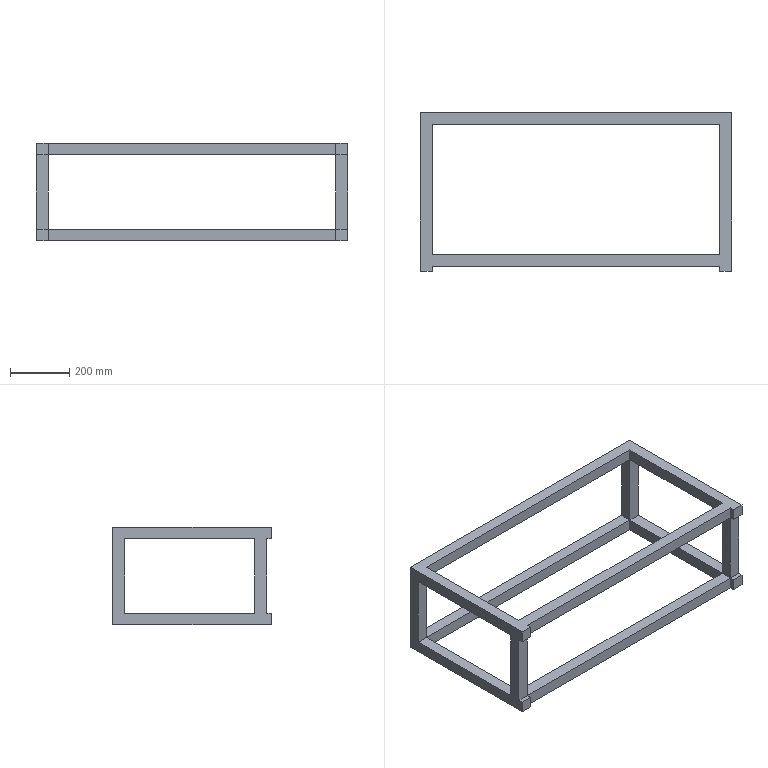Part | NX | 1 solid | 45 faces | box 1050 x 535 x 330 mm | volume 11232000 mm3 | plane 45
STEP:
#1=CARTESIAN_POINT('',(485.,-20.,165.));
#2=VERTEX_POINT('',#1);
#3=CARTESIAN_POINT('',(485.,-20.,125.));
#4=VERTEX_POINT('',#3);
#5=CARTESIAN_POINT('',(485.,-20.,165.));
#6=DIRECTION('',(0.,0.,-1.));
#7=VECTOR('',#6,1.);
#8=LINE('',#5,#7);
#9=EDGE_CURVE('',#2,#4,#8,.T.);
#10=ORIENTED_EDGE('',*,*,#9,.F.);
#11=CARTESIAN_POINT('',(-485.,-20.,165.));
#12=VERTEX_POINT('',#11);
#13=CARTESIAN_POINT('',(-485.,-20.,165.));
#14=DIRECTION('',(1.,0.,0.));
#15=VECTOR('',#14,1.);
#16=LINE('',#13,#15);
#17=EDGE_CURVE('',#12,#2,#16,.T.);
#18=ORIENTED_EDGE('',*,*,#17,.F.);
#19=CARTESIAN_POINT('',(-485.,-20.,125.));
#20=VERTEX_POINT('',#19);
#21=CARTESIAN_POINT('',(-485.,-20.,165.));
#22=DIRECTION('',(0.,0.,-1.));
#23=VECTOR('',#22,1.);
#24=LINE('',#21,#23);
#25=EDGE_CURVE('',#12,#20,#24,.T.);
#26=ORIENTED_EDGE('',*,*,#25,.T.);
#27=CARTESIAN_POINT('',(485.,-20.,125.));
#28=DIRECTION('',(-1.,0.,0.));
#29=VECTOR('',#28,1.);
#30=LINE('',#27,#29);
#31=EDGE_CURVE('',#4,#20,#30,.T.);
#32=ORIENTED_EDGE('',*,*,#31,.F.);
#33=EDGE_LOOP('',(#10,#18,#26,#32));
#34=FACE_OUTER_BOUND('',#33,.T.);
#35=CARTESIAN_POINT('',(0.,-20.,0.));
#36=DIRECTION('',(0.,1.,0.));
#37=DIRECTION('',(0.,0.,1.));
#38=AXIS2_PLACEMENT_3D('',#35,#36,#37);
#39=PLANE('',#38);
#40=ADVANCED_FACE('',(#34),#39,.F.);
#41=CARTESIAN_POINT('',(525.,-20.,125.));
#42=VERTEX_POINT('',#41);
#43=CARTESIAN_POINT('',(525.,-20.,125.));
#44=DIRECTION('',(-1.,0.,0.));
#45=VECTOR('',#44,1.);
#46=LINE('',#43,#45);
#47=EDGE_CURVE('',#42,#4,#46,.T.);
#48=ORIENTED_EDGE('',*,*,#47,.T.);
#49=CARTESIAN_POINT('',(485.,-20.,-125.));
#50=VERTEX_POINT('',#49);
#51=CARTESIAN_POINT('',(485.,-20.,-125.));
#52=DIRECTION('',(0.,0.,1.));
#53=VECTOR('',#52,1.);
#54=LINE('',#51,#53);
#55=EDGE_CURVE('',#50,#4,#54,.T.);
#56=ORIENTED_EDGE('',*,*,#55,.F.);
#57=CARTESIAN_POINT('',(525.,-20.,-125.));
#58=VERTEX_POINT('',#57);
#59=CARTESIAN_POINT('',(525.,-20.,-125.));
#60=DIRECTION('',(-1.,0.,0.));
#61=VECTOR('',#60,1.);
#62=LINE('',#59,#61);
#63=EDGE_CURVE('',#58,#50,#62,.T.);
#64=ORIENTED_EDGE('',*,*,#63,.F.);
#65=CARTESIAN_POINT('',(525.,-20.,125.));
#66=DIRECTION('',(0.,0.,-1.));
#67=VECTOR('',#66,1.);
#68=LINE('',#65,#67);
#69=EDGE_CURVE('',#42,#58,#68,.T.);
#70=ORIENTED_EDGE('',*,*,#69,.F.);
#71=EDGE_LOOP('',(#48,#56,#64,#70));
#72=FACE_OUTER_BOUND('',#71,.T.);
#73=CARTESIAN_POINT('',(0.,-20.,0.));
#74=DIRECTION('',(0.,1.,0.));
#75=DIRECTION('',(0.,0.,1.));
#76=AXIS2_PLACEMENT_3D('',#73,#74,#75);
#77=PLANE('',#76);
#78=ADVANCED_FACE('',(#72),#77,.F.);
#79=CARTESIAN_POINT('',(485.,-20.,-165.));
#80=VERTEX_POINT('',#79);
#81=CARTESIAN_POINT('',(485.,-20.,-165.));
#82=DIRECTION('',(0.,0.,1.));
#83=VECTOR('',#82,1.);
#84=LINE('',#81,#83);
#85=EDGE_CURVE('',#80,#50,#84,.T.);
#86=ORIENTED_EDGE('',*,*,#85,.T.);
#87=CARTESIAN_POINT('',(-485.,-20.,-125.));
#88=VERTEX_POINT('',#87);
#89=CARTESIAN_POINT('',(-485.,-20.,-125.));
#90=DIRECTION('',(1.,0.,0.));
#91=VECTOR('',#90,1.);
#92=LINE('',#89,#91);
#93=EDGE_CURVE('',#88,#50,#92,.T.);
#94=ORIENTED_EDGE('',*,*,#93,.F.);
#95=CARTESIAN_POINT('',(-485.,-20.,-165.));
#96=VERTEX_POINT('',#95);
#97=CARTESIAN_POINT('',(-485.,-20.,-165.));
#98=DIRECTION('',(0.,0.,1.));
#99=VECTOR('',#98,1.);
#100=LINE('',#97,#99);
#101=EDGE_CURVE('',#96,#88,#100,.T.);
#102=ORIENTED_EDGE('',*,*,#101,.F.);
#103=CARTESIAN_POINT('',(485.,-20.,-165.));
#104=DIRECTION('',(-1.,0.,0.));
#105=VECTOR('',#104,1.);
#106=LINE('',#103,#105);
#107=EDGE_CURVE('',#80,#96,#106,.T.);
#108=ORIENTED_EDGE('',*,*,#107,.F.);
#109=EDGE_LOOP('',(#86,#94,#102,#108));
#110=FACE_OUTER_BOUND('',#109,.T.);
#111=CARTESIAN_POINT('',(0.,-20.,0.));
#112=DIRECTION('',(0.,1.,0.));
#113=DIRECTION('',(0.,0.,1.));
#114=AXIS2_PLACEMENT_3D('',#111,#112,#113);
#115=PLANE('',#114);
#116=ADVANCED_FACE('',(#110),#115,.F.);
#117=CARTESIAN_POINT('',(-525.,-20.,-125.));
#118=VERTEX_POINT('',#117);
#119=CARTESIAN_POINT('',(-525.,-20.,-125.));
#120=DIRECTION('',(1.,0.,0.));
#121=VECTOR('',#120,1.);
#122=LINE('',#119,#121);
#123=EDGE_CURVE('',#118,#88,#122,.T.);
#124=ORIENTED_EDGE('',*,*,#123,.T.);
#125=CARTESIAN_POINT('',(-485.,-20.,125.));
#126=DIRECTION('',(0.,0.,-1.));
#127=VECTOR('',#126,1.);
#128=LINE('',#125,#127);
#129=EDGE_CURVE('',#20,#88,#128,.T.);
#130=ORIENTED_EDGE('',*,*,#129,.F.);
#131=CARTESIAN_POINT('',(-525.,-20.,125.));
#132=VERTEX_POINT('',#131);
#133=CARTESIAN_POINT('',(-525.,-20.,125.));
#134=DIRECTION('',(1.,0.,0.));
#135=VECTOR('',#134,1.);
#136=LINE('',#133,#135);
#137=EDGE_CURVE('',#132,#20,#136,.T.);
#138=ORIENTED_EDGE('',*,*,#137,.F.);
#139=CARTESIAN_POINT('',(-525.,-20.,-125.));
#140=DIRECTION('',(0.,0.,1.));
#141=VECTOR('',#140,1.);
#142=LINE('',#139,#141);
#143=EDGE_CURVE('',#118,#132,#142,.T.);
#144=ORIENTED_EDGE('',*,*,#143,.F.);
#145=EDGE_LOOP('',(#124,#130,#138,#144));
#146=FACE_OUTER_BOUND('',#145,.T.);
#147=CARTESIAN_POINT('',(0.,-20.,0.));
#148=DIRECTION('',(0.,1.,0.));
#149=DIRECTION('',(0.,0.,1.));
#150=AXIS2_PLACEMENT_3D('',#147,#148,#149);
#151=PLANE('',#150);
#152=ADVANCED_FACE('',(#146),#151,.F.);
#153=CARTESIAN_POINT('',(-525.,20.,-165.));
#154=VERTEX_POINT('',#153);
#155=CARTESIAN_POINT('',(-525.,20.,165.));
#156=VERTEX_POINT('',#155);
#157=CARTESIAN_POINT('',(-525.,20.,-165.));
#158=DIRECTION('',(0.,0.,1.));
#159=VECTOR('',#158,1.);
#160=LINE('',#157,#159);
#161=EDGE_CURVE('',#154,#156,#160,.T.);
#162=ORIENTED_EDGE('',*,*,#161,.T.);
#163=CARTESIAN_POINT('',(525.,20.,165.));
#164=VERTEX_POINT('',#163);
#165=CARTESIAN_POINT('',(-525.,20.,165.));
#166=DIRECTION('',(1.,0.,0.));
#167=VECTOR('',#166,1.);
#168=LINE('',#165,#167);
#169=EDGE_CURVE('',#156,#164,#168,.T.);
#170=ORIENTED_EDGE('',*,*,#169,.T.);
#171=CARTESIAN_POINT('',(525.,20.,-165.));
#172=VERTEX_POINT('',#171);
#173=CARTESIAN_POINT('',(525.,20.,165.));
#174=DIRECTION('',(0.,0.,-1.));
#175=VECTOR('',#174,1.);
#176=LINE('',#173,#175);
#177=EDGE_CURVE('',#164,#172,#176,.T.);
#178=ORIENTED_EDGE('',*,*,#177,.T.);
#179=CARTESIAN_POINT('',(525.,20.,-165.));
#180=DIRECTION('',(-1.,0.,0.));
#181=VECTOR('',#180,1.);
#182=LINE('',#179,#181);
#183=EDGE_CURVE('',#172,#154,#182,.T.);
#184=ORIENTED_EDGE('',*,*,#183,.T.);
#185=EDGE_LOOP('',(#162,#170,#178,#184));
#186=FACE_BOUND('',#185,.T.);
#187=CARTESIAN_POINT('',(-485.,20.,-125.));
#188=VERTEX_POINT('',#187);
#189=CARTESIAN_POINT('',(485.,20.,-125.));
#190=VERTEX_POINT('',#189);
#191=CARTESIAN_POINT('',(-485.,20.,-125.));
#192=DIRECTION('',(1.,0.,0.));
#193=VECTOR('',#192,1.);
#194=LINE('',#191,#193);
#195=EDGE_CURVE('',#188,#190,#194,.T.);
#196=ORIENTED_EDGE('',*,*,#195,.T.);
#197=CARTESIAN_POINT('',(485.,20.,125.));
#198=VERTEX_POINT('',#197);
#199=CARTESIAN_POINT('',(485.,20.,-125.));
#200=DIRECTION('',(0.,0.,1.));
#201=VECTOR('',#200,1.);
#202=LINE('',#199,#201);
#203=EDGE_CURVE('',#190,#198,#202,.T.);
#204=ORIENTED_EDGE('',*,*,#203,.T.);
#205=CARTESIAN_POINT('',(-485.,20.,125.));
#206=VERTEX_POINT('',#205);
#207=CARTESIAN_POINT('',(485.,20.,125.));
#208=DIRECTION('',(-1.,0.,0.));
#209=VECTOR('',#208,1.);
#210=LINE('',#207,#209);
#211=EDGE_CURVE('',#198,#206,#210,.T.);
#212=ORIENTED_EDGE('',*,*,#211,.T.);
#213=CARTESIAN_POINT('',(-485.,20.,125.));
#214=DIRECTION('',(0.,0.,-1.));
#215=VECTOR('',#214,1.);
#216=LINE('',#213,#215);
#217=EDGE_CURVE('',#206,#188,#216,.T.);
#218=ORIENTED_EDGE('',*,*,#217,.T.);
#219=EDGE_LOOP('',(#196,#204,#212,#218));
#220=FACE_BOUND('',#219,.T.);
#221=CARTESIAN_POINT('',(0.,20.,0.));
#222=DIRECTION('',(0.,1.,0.));
#223=DIRECTION('',(0.,0.,1.));
#224=AXIS2_PLACEMENT_3D('',#221,#222,#223);
#225=PLANE('',#224);
#226=ADVANCED_FACE('',(#186,#220),#225,.T.);
#227=CARTESIAN_POINT('',(-525.,-500.,125.));
#228=VERTEX_POINT('',#227);
#229=CARTESIAN_POINT('',(-525.,-515.,125.));
#230=VERTEX_POINT('',#229);
#231=CARTESIAN_POINT('',(-525.,-500.,125.));
#232=DIRECTION('',(0.,-1.,0.));
#233=VECTOR('',#232,1.);
#234=LINE('',#231,#233);
#235=EDGE_CURVE('',#228,#230,#234,.T.);
#236=ORIENTED_EDGE('',*,*,#235,.T.);
#237=CARTESIAN_POINT('',(-525.,-515.,165.));
#238=VERTEX_POINT('',#237);
#239=CARTESIAN_POINT('',(-525.,-515.,165.));
#240=DIRECTION('',(0.,0.,-1.));
#241=VECTOR('',#240,1.);
#242=LINE('',#239,#241);
#243=EDGE_CURVE('',#238,#230,#242,.T.);
#244=ORIENTED_EDGE('',*,*,#243,.F.);
#245=CARTESIAN_POINT('',(-525.,20.,165.));
#246=DIRECTION('',(0.,-1.,0.));
#247=VECTOR('',#246,1.);
#248=LINE('',#245,#247);
#249=EDGE_CURVE('',#156,#238,#248,.T.);
#250=ORIENTED_EDGE('',*,*,#249,.F.);
#251=ORIENTED_EDGE('',*,*,#161,.F.);
#252=CARTESIAN_POINT('',(-525.,-515.,-165.));
#253=VERTEX_POINT('',#252);
#254=CARTESIAN_POINT('',(-525.,-515.,-165.));
#255=DIRECTION('',(0.,1.,0.));
#256=VECTOR('',#255,1.);
#257=LINE('',#254,#256);
#258=EDGE_CURVE('',#253,#154,#257,.T.);
#259=ORIENTED_EDGE('',*,*,#258,.F.);
#260=CARTESIAN_POINT('',(-525.,-515.,-125.));
#261=VERTEX_POINT('',#260);
#262=CARTESIAN_POINT('',(-525.,-515.,-125.));
#263=DIRECTION('',(0.,0.,-1.));
#264=VECTOR('',#263,1.);
#265=LINE('',#262,#264);
#266=EDGE_CURVE('',#261,#253,#265,.T.);
#267=ORIENTED_EDGE('',*,*,#266,.F.);
#268=CARTESIAN_POINT('',(-525.,-500.,-125.));
#269=VERTEX_POINT('',#268);
#270=CARTESIAN_POINT('',(-525.,-500.,-125.));
#271=DIRECTION('',(0.,-1.,0.));
#272=VECTOR('',#271,1.);
#273=LINE('',#270,#272);
#274=EDGE_CURVE('',#269,#261,#273,.T.);
#275=ORIENTED_EDGE('',*,*,#274,.F.);
#276=CARTESIAN_POINT('',(-525.,-500.,125.));
#277=DIRECTION('',(0.,0.,-1.));
#278=VECTOR('',#277,1.);
#279=LINE('',#276,#278);
#280=EDGE_CURVE('',#228,#269,#279,.T.);
#281=ORIENTED_EDGE('',*,*,#280,.F.);
#282=EDGE_LOOP('',(#236,#244,#250,#251,#259,#267,#275,#281));
#283=FACE_BOUND('',#282,.T.);
#284=CARTESIAN_POINT('',(-525.,-460.,-125.));
#285=VERTEX_POINT('',#284);
#286=CARTESIAN_POINT('',(-525.,-20.,-125.));
#287=DIRECTION('',(0.,-1.,0.));
#288=VECTOR('',#287,1.);
#289=LINE('',#286,#288);
#290=EDGE_CURVE('',#118,#285,#289,.T.);
#291=ORIENTED_EDGE('',*,*,#290,.F.);
#292=ORIENTED_EDGE('',*,*,#143,.T.);
#293=CARTESIAN_POINT('',(-525.,-460.,125.));
#294=VERTEX_POINT('',#293);
#295=CARTESIAN_POINT('',(-525.,-20.,125.));
#296=DIRECTION('',(0.,-1.,0.));
#297=VECTOR('',#296,1.);
#298=LINE('',#295,#297);
#299=EDGE_CURVE('',#132,#294,#298,.T.);
#300=ORIENTED_EDGE('',*,*,#299,.T.);
#301=CARTESIAN_POINT('',(-525.,-460.,125.));
#302=DIRECTION('',(0.,0.,-1.));
#303=VECTOR('',#302,1.);
#304=LINE('',#301,#303);
#305=EDGE_CURVE('',#294,#285,#304,.T.);
#306=ORIENTED_EDGE('',*,*,#305,.T.);
#307=EDGE_LOOP('',(#291,#292,#300,#306));
#308=FACE_BOUND('',#307,.T.);
#309=CARTESIAN_POINT('',(-525.,-20.,-165.));
#310=DIRECTION('',(-1.,0.,0.));
#311=DIRECTION('',(0.,0.,1.));
#312=AXIS2_PLACEMENT_3D('',#309,#310,#311);
#313=PLANE('',#312);
#314=ADVANCED_FACE('',(#283,#308),#313,.T.);
#315=CARTESIAN_POINT('',(485.,-500.,165.));
#316=VERTEX_POINT('',#315);
#317=CARTESIAN_POINT('',(485.,-515.,165.));
#318=VERTEX_POINT('',#317);
#319=CARTESIAN_POINT('',(485.,-500.,165.));
#320=DIRECTION('',(0.,-1.,0.));
#321=VECTOR('',#320,1.);
#322=LINE('',#319,#321);
#323=EDGE_CURVE('',#316,#318,#322,.T.);
#324=ORIENTED_EDGE('',*,*,#323,.T.);
#325=CARTESIAN_POINT('',(525.,-515.,165.));
#326=VERTEX_POINT('',#325);
#327=CARTESIAN_POINT('',(525.,-515.,165.));
#328=DIRECTION('',(-1.,0.,0.));
#329=VECTOR('',#328,1.);
#330=LINE('',#327,#329);
#331=EDGE_CURVE('',#326,#318,#330,.T.);
#332=ORIENTED_EDGE('',*,*,#331,.F.);
#333=CARTESIAN_POINT('',(525.,20.,165.));
#334=DIRECTION('',(0.,-1.,0.));
#335=VECTOR('',#334,1.);
#336=LINE('',#333,#335);
#337=EDGE_CURVE('',#164,#326,#336,.T.);
#338=ORIENTED_EDGE('',*,*,#337,.F.);
#339=ORIENTED_EDGE('',*,*,#169,.F.);
#340=ORIENTED_EDGE('',*,*,#249,.T.);
#341=CARTESIAN_POINT('',(-485.,-515.,165.));
#342=VERTEX_POINT('',#341);
#343=CARTESIAN_POINT('',(-485.,-515.,165.));
#344=DIRECTION('',(-1.,0.,0.));
#345=VECTOR('',#344,1.);
#346=LINE('',#343,#345);
#347=EDGE_CURVE('',#342,#238,#346,.T.);
#348=ORIENTED_EDGE('',*,*,#347,.F.);
#349=CARTESIAN_POINT('',(-485.,-500.,165.));
#350=VERTEX_POINT('',#349);
#351=CARTESIAN_POINT('',(-485.,-500.,165.));
#352=DIRECTION('',(0.,-1.,0.));
#353=VECTOR('',#352,1.);
#354=LINE('',#351,#353);
#355=EDGE_CURVE('',#350,#342,#354,.T.);
#356=ORIENTED_EDGE('',*,*,#355,.F.);
#357=CARTESIAN_POINT('',(485.,-500.,165.));
#358=DIRECTION('',(-1.,0.,0.));
#359=VECTOR('',#358,1.);
#360=LINE('',#357,#359);
#361=EDGE_CURVE('',#316,#350,#360,.T.);
#362=ORIENTED_EDGE('',*,*,#361,.F.);
#363=EDGE_LOOP('',(#324,#332,#338,#339,#340,#348,#356,#362));
#364=FACE_BOUND('',#363,.T.);
#365=CARTESIAN_POINT('',(-485.,-460.,165.));
#366=VERTEX_POINT('',#365);
#367=CARTESIAN_POINT('',(-485.,-20.,165.));
#368=DIRECTION('',(0.,-1.,0.));
#369=VECTOR('',#368,1.);
#370=LINE('',#367,#369);
#371=EDGE_CURVE('',#12,#366,#370,.T.);
#372=ORIENTED_EDGE('',*,*,#371,.F.);
#373=ORIENTED_EDGE('',*,*,#17,.T.);
#374=CARTESIAN_POINT('',(485.,-460.,165.));
#375=VERTEX_POINT('',#374);
#376=CARTESIAN_POINT('',(485.,-20.,165.));
#377=DIRECTION('',(0.,-1.,0.));
#378=VECTOR('',#377,1.);
#379=LINE('',#376,#378);
#380=EDGE_CURVE('',#2,#375,#379,.T.);
#381=ORIENTED_EDGE('',*,*,#380,.T.);
#382=CARTESIAN_POINT('',(485.,-460.,165.));
#383=DIRECTION('',(-1.,0.,0.));
#384=VECTOR('',#383,1.);
#385=LINE('',#382,#384);
#386=EDGE_CURVE('',#375,#366,#385,.T.);
#387=ORIENTED_EDGE('',*,*,#386,.T.);
#388=EDGE_LOOP('',(#372,#373,#381,#387));
#389=FACE_BOUND('',#388,.T.);
#390=CARTESIAN_POINT('',(-525.,-20.,165.));
#391=DIRECTION('',(0.,0.,1.));
#392=DIRECTION('',(1.,0.,0.));
#393=AXIS2_PLACEMENT_3D('',#390,#391,#392);
#394=PLANE('',#393);
#395=ADVANCED_FACE('',(#364,#389),#394,.T.);
#396=CARTESIAN_POINT('',(525.,-500.,-125.));
#397=VERTEX_POINT('',#396);
#398=CARTESIAN_POINT('',(525.,-515.,-125.));
#399=VERTEX_POINT('',#398);
#400=CARTESIAN_POINT('',(525.,-500.,-125.));
#401=DIRECTION('',(0.,-1.,0.));
#402=VECTOR('',#401,1.);
#403=LINE('',#400,#402);
#404=EDGE_CURVE('',#397,#399,#403,.T.);
#405=ORIENTED_EDGE('',*,*,#404,.T.);
#406=CARTESIAN_POINT('',(525.,-515.,-165.));
#407=VERTEX_POINT('',#406);
#408=CARTESIAN_POINT('',(525.,-515.,-165.));
#409=DIRECTION('',(0.,0.,1.));
#410=VECTOR('',#409,1.);
#411=LINE('',#408,#410);
#412=EDGE_CURVE('',#407,#399,#411,.T.);
#413=ORIENTED_EDGE('',*,*,#412,.F.);
#414=CARTESIAN_POINT('',(525.,-515.,-165.));
#415=DIRECTION('',(0.,1.,0.));
#416=VECTOR('',#415,1.);
#417=LINE('',#414,#416);
#418=EDGE_CURVE('',#407,#172,#417,.T.);
#419=ORIENTED_EDGE('',*,*,#418,.T.);
#420=ORIENTED_EDGE('',*,*,#177,.F.);
#421=ORIENTED_EDGE('',*,*,#337,.T.);
#422=CARTESIAN_POINT('',(525.,-515.,125.));
#423=VERTEX_POINT('',#422);
#424=CARTESIAN_POINT('',(525.,-515.,125.));
#425=DIRECTION('',(0.,0.,1.));
#426=VECTOR('',#425,1.);
#427=LINE('',#424,#426);
#428=EDGE_CURVE('',#423,#326,#427,.T.);
#429=ORIENTED_EDGE('',*,*,#428,.F.);
#430=CARTESIAN_POINT('',(525.,-500.,125.));
#431=VERTEX_POINT('',#430);
#432=CARTESIAN_POINT('',(525.,-500.,125.));
#433=DIRECTION('',(0.,-1.,0.));
#434=VECTOR('',#433,1.);
#435=LINE('',#432,#434);
#436=EDGE_CURVE('',#431,#423,#435,.T.);
#437=ORIENTED_EDGE('',*,*,#436,.F.);
#438=CARTESIAN_POINT('',(525.,-500.,-125.));
#439=DIRECTION('',(0.,0.,1.));
#440=VECTOR('',#439,1.);
#441=LINE('',#438,#440);
#442=EDGE_CURVE('',#397,#431,#441,.T.);
#443=ORIENTED_EDGE('',*,*,#442,.F.);
#444=EDGE_LOOP('',(#405,#413,#419,#420,#421,#429,#437,#443));
#445=FACE_BOUND('',#444,.T.);
#446=CARTESIAN_POINT('',(525.,-460.,125.));
#447=VERTEX_POINT('',#446);
#448=CARTESIAN_POINT('',(525.,-20.,125.));
#449=DIRECTION('',(0.,-1.,0.));
#450=VECTOR('',#449,1.);
#451=LINE('',#448,#450);
#452=EDGE_CURVE('',#42,#447,#451,.T.);
#453=ORIENTED_EDGE('',*,*,#452,.F.);
#454=ORIENTED_EDGE('',*,*,#69,.T.);
#455=CARTESIAN_POINT('',(525.,-460.,-125.));
#456=VERTEX_POINT('',#455);
#457=CARTESIAN_POINT('',(525.,-20.,-125.));
#458=DIRECTION('',(0.,-1.,0.));
#459=VECTOR('',#458,1.);
#460=LINE('',#457,#459);
#461=EDGE_CURVE('',#58,#456,#460,.T.);
#462=ORIENTED_EDGE('',*,*,#461,.T.);
#463=CARTESIAN_POINT('',(525.,-460.,-125.));
#464=DIRECTION('',(0.,0.,1.));
#465=VECTOR('',#464,1.);
#466=LINE('',#463,#465);
#467=EDGE_CURVE('',#456,#447,#466,.T.);
#468=ORIENTED_EDGE('',*,*,#467,.T.);
#469=EDGE_LOOP('',(#453,#454,#462,#468));
#470=FACE_BOUND('',#469,.T.);
#471=CARTESIAN_POINT('',(525.,-20.,165.));
#472=DIRECTION('',(1.,0.,0.));
#473=DIRECTION('',(0.,0.,-1.));
#474=AXIS2_PLACEMENT_3D('',#471,#472,#473);
#475=PLANE('',#474);
#476=ADVANCED_FACE('',(#445,#470),#475,.T.);
#477=CARTESIAN_POINT('',(-485.,-500.,-165.));
#478=VERTEX_POINT('',#477);
#479=CARTESIAN_POINT('',(-485.,-515.,-165.));
#480=VERTEX_POINT('',#479);
#481=CARTESIAN_POINT('',(-485.,-500.,-165.));
#482=DIRECTION('',(0.,-1.,0.));
#483=VECTOR('',#482,1.);
#484=LINE('',#481,#483);
#485=EDGE_CURVE('',#478,#480,#484,.T.);
#486=ORIENTED_EDGE('',*,*,#485,.T.);
#487=CARTESIAN_POINT('',(-525.,-515.,-165.));
#488=DIRECTION('',(1.,0.,0.));
#489=VECTOR('',#488,1.);
#490=LINE('',#487,#489);
#491=EDGE_CURVE('',#253,#480,#490,.T.);
#492=ORIENTED_EDGE('',*,*,#491,.F.);
#493=ORIENTED_EDGE('',*,*,#258,.T.);
#494=ORIENTED_EDGE('',*,*,#183,.F.);
#495=ORIENTED_EDGE('',*,*,#418,.F.);
#496=CARTESIAN_POINT('',(485.,-515.,-165.));
#497=VERTEX_POINT('',#496);
#498=CARTESIAN_POINT('',(485.,-515.,-165.));
#499=DIRECTION('',(1.,0.,0.));
#500=VECTOR('',#499,1.);
#501=LINE('',#498,#500);
#502=EDGE_CURVE('',#497,#407,#501,.T.);
#503=ORIENTED_EDGE('',*,*,#502,.F.);
#504=CARTESIAN_POINT('',(485.,-500.,-165.));
#505=VERTEX_POINT('',#504);
#506=CARTESIAN_POINT('',(485.,-500.,-165.));
#507=DIRECTION('',(0.,-1.,0.));
#508=VECTOR('',#507,1.);
#509=LINE('',#506,#508);
#510=EDGE_CURVE('',#505,#497,#509,.T.);
#511=ORIENTED_EDGE('',*,*,#510,.F.);
#512=CARTESIAN_POINT('',(485.,-500.,-165.));
#513=DIRECTION('',(-1.,0.,0.));
#514=VECTOR('',#513,1.);
#515=LINE('',#512,#514);
#516=EDGE_CURVE('',#505,#478,#515,.T.);
#517=ORIENTED_EDGE('',*,*,#516,.T.);
#518=EDGE_LOOP('',(#486,#492,#493,#494,#495,#503,#511,#517));
#519=FACE_BOUND('',#518,.T.);
#520=CARTESIAN_POINT('',(485.,-460.,-165.));
#521=VERTEX_POINT('',#520);
#522=CARTESIAN_POINT('',(485.,-20.,-165.));
#523=DIRECTION('',(0.,-1.,0.));
#524=VECTOR('',#523,1.);
#525=LINE('',#522,#524);
#526=EDGE_CURVE('',#80,#521,#525,.T.);
#527=ORIENTED_EDGE('',*,*,#526,.F.);
#528=ORIENTED_EDGE('',*,*,#107,.T.);
#529=CARTESIAN_POINT('',(-485.,-460.,-165.));
#530=VERTEX_POINT('',#529);
#531=CARTESIAN_POINT('',(-485.,-20.,-165.));
#532=DIRECTION('',(0.,-1.,0.));
#533=VECTOR('',#532,1.);
#534=LINE('',#531,#533);
#535=EDGE_CURVE('',#96,#530,#534,.T.);
#536=ORIENTED_EDGE('',*,*,#535,.T.);
#537=CARTESIAN_POINT('',(485.,-460.,-165.));
#538=DIRECTION('',(-1.,0.,0.));
#539=VECTOR('',#538,1.);
#540=LINE('',#537,#539);
#541=EDGE_CURVE('',#521,#530,#540,.T.);
#542=ORIENTED_EDGE('',*,*,#541,.F.);
#543=EDGE_LOOP('',(#527,#528,#536,#542));
#544=FACE_BOUND('',#543,.T.);
#545=CARTESIAN_POINT('',(525.,-20.,-165.));
#546=DIRECTION('',(0.,0.,-1.));
#547=DIRECTION('',(-1.,0.,0.));
#548=AXIS2_PLACEMENT_3D('',#545,#546,#547);
#549=PLANE('',#548);
#550=ADVANCED_FACE('',(#519,#544),#549,.T.);
#551=ORIENTED_EDGE('',*,*,#93,.T.);
#552=CARTESIAN_POINT('',(485.,-20.,-125.));
#553=DIRECTION('',(0.,1.,0.));
#554=VECTOR('',#553,1.);
#555=LINE('',#552,#554);
#556=EDGE_CURVE('',#50,#190,#555,.T.);
#557=ORIENTED_EDGE('',*,*,#556,.T.);
#558=ORIENTED_EDGE('',*,*,#195,.F.);
#559=CARTESIAN_POINT('',(-485.,-20.,-125.));
#560=DIRECTION('',(0.,1.,0.));
#561=VECTOR('',#560,1.);
#562=LINE('',#559,#561);
#563=EDGE_CURVE('',#88,#188,#562,.T.);
#564=ORIENTED_EDGE('',*,*,#563,.F.);
#565=EDGE_LOOP('',(#551,#557,#558,#564));
#566=FACE_OUTER_BOUND('',#565,.T.);
#567=CARTESIAN_POINT('',(-485.,-20.,-125.));
#568=DIRECTION('',(0.,0.,1.));
#569=DIRECTION('',(1.,0.,0.));
#570=AXIS2_PLACEMENT_3D('',#567,#568,#569);
#571=PLANE('',#570);
#572=ADVANCED_FACE('',(#566),#571,.T.);
#573=ORIENTED_EDGE('',*,*,#55,.T.);
#574=CARTESIAN_POINT('',(485.,-20.,125.));
#575=DIRECTION('',(0.,1.,0.));
#576=VECTOR('',#575,1.);
#577=LINE('',#574,#576);
#578=EDGE_CURVE('',#4,#198,#577,.T.);
#579=ORIENTED_EDGE('',*,*,#578,.T.);
#580=ORIENTED_EDGE('',*,*,#203,.F.);
#581=ORIENTED_EDGE('',*,*,#556,.F.);
#582=EDGE_LOOP('',(#573,#579,#580,#581));
#583=FACE_OUTER_BOUND('',#582,.T.);
#584=CARTESIAN_POINT('',(485.,-20.,-125.));
#585=DIRECTION('',(-1.,0.,0.));
#586=DIRECTION('',(0.,0.,1.));
#587=AXIS2_PLACEMENT_3D('',#584,#585,#586);
#588=PLANE('',#587);
#589=ADVANCED_FACE('',(#583),#588,.T.);
#590=ORIENTED_EDGE('',*,*,#31,.T.);
#591=CARTESIAN_POINT('',(-485.,-20.,125.));
#592=DIRECTION('',(0.,1.,0.));
#593=VECTOR('',#592,1.);
#594=LINE('',#591,#593);
#595=EDGE_CURVE('',#20,#206,#594,.T.);
#596=ORIENTED_EDGE('',*,*,#595,.T.);
#597=ORIENTED_EDGE('',*,*,#211,.F.);
#598=ORIENTED_EDGE('',*,*,#578,.F.);
#599=EDGE_LOOP('',(#590,#596,#597,#598));
#600=FACE_OUTER_BOUND('',#599,.T.);
#601=CARTESIAN_POINT('',(485.,-20.,125.));
#602=DIRECTION('',(0.,0.,-1.));
#603=DIRECTION('',(-1.,0.,0.));
#604=AXIS2_PLACEMENT_3D('',#601,#602,#603);
#605=PLANE('',#604);
#606=ADVANCED_FACE('',(#600),#605,.T.);
#607=ORIENTED_EDGE('',*,*,#129,.T.);
#608=ORIENTED_EDGE('',*,*,#563,.T.);
#609=ORIENTED_EDGE('',*,*,#217,.F.);
#610=ORIENTED_EDGE('',*,*,#595,.F.);
#611=EDGE_LOOP('',(#607,#608,#609,#610));
#612=FACE_OUTER_BOUND('',#611,.T.);
#613=CARTESIAN_POINT('',(-485.,-20.,125.));
#614=DIRECTION('',(1.,0.,0.));
#615=DIRECTION('',(0.,0.,-1.));
#616=AXIS2_PLACEMENT_3D('',#613,#614,#615);
#617=PLANE('',#616);
#618=ADVANCED_FACE('',(#612),#617,.T.);
#619=CARTESIAN_POINT('',(485.,-515.,125.));
#620=VERTEX_POINT('',#619);
#621=CARTESIAN_POINT('',(485.,-515.,165.));
#622=DIRECTION('',(0.,0.,-1.));
#623=VECTOR('',#622,1.);
#624=LINE('',#621,#623);
#625=EDGE_CURVE('',#318,#620,#624,.T.);
#626=ORIENTED_EDGE('',*,*,#625,.T.);
#627=CARTESIAN_POINT('',(485.,-515.,125.));
#628=DIRECTION('',(1.,0.,0.));
#629=VECTOR('',#628,1.);
#630=LINE('',#627,#629);
#631=EDGE_CURVE('',#620,#423,#630,.T.);
#632=ORIENTED_EDGE('',*,*,#631,.T.);
#633=ORIENTED_EDGE('',*,*,#428,.T.);
#634=ORIENTED_EDGE('',*,*,#331,.T.);
#635=EDGE_LOOP('',(#626,#632,#633,#634));
#636=FACE_OUTER_BOUND('',#635,.T.);
#637=CARTESIAN_POINT('',(0.,-515.,0.));
#638=DIRECTION('',(0.,-1.,0.));
#639=DIRECTION('',(0.,0.,-1.));
#640=AXIS2_PLACEMENT_3D('',#637,#638,#639);
#641=PLANE('',#640);
#642=ADVANCED_FACE('',(#636),#641,.T.);
#643=CARTESIAN_POINT('',(485.,-515.,-125.));
#644=VERTEX_POINT('',#643);
#645=CARTESIAN_POINT('',(485.,-515.,-125.));
#646=DIRECTION('',(0.,0.,-1.));
#647=VECTOR('',#646,1.);
#648=LINE('',#645,#647);
#649=EDGE_CURVE('',#644,#497,#648,.T.);
#650=ORIENTED_EDGE('',*,*,#649,.T.);
#651=ORIENTED_EDGE('',*,*,#502,.T.);
#652=ORIENTED_EDGE('',*,*,#412,.T.);
#653=CARTESIAN_POINT('',(525.,-515.,-125.));
#654=DIRECTION('',(-1.,0.,0.));
#655=VECTOR('',#654,1.);
#656=LINE('',#653,#655);
#657=EDGE_CURVE('',#399,#644,#656,.T.);
#658=ORIENTED_EDGE('',*,*,#657,.T.);
#659=EDGE_LOOP('',(#650,#651,#652,#658));
#660=FACE_OUTER_BOUND('',#659,.T.);
#661=CARTESIAN_POINT('',(0.,-515.,0.));
#662=DIRECTION('',(0.,-1.,0.));
#663=DIRECTION('',(0.,0.,-1.));
#664=AXIS2_PLACEMENT_3D('',#661,#662,#663);
#665=PLANE('',#664);
#666=ADVANCED_FACE('',(#660),#665,.T.);
#667=ORIENTED_EDGE('',*,*,#266,.T.);
#668=ORIENTED_EDGE('',*,*,#491,.T.);
#669=CARTESIAN_POINT('',(-485.,-515.,-125.));
#670=VERTEX_POINT('',#669);
#671=CARTESIAN_POINT('',(-485.,-515.,-165.));
#672=DIRECTION('',(0.,0.,1.));
#673=VECTOR('',#672,1.);
#674=LINE('',#671,#673);
#675=EDGE_CURVE('',#480,#670,#674,.T.);
#676=ORIENTED_EDGE('',*,*,#675,.T.);
#677=CARTESIAN_POINT('',(-485.,-515.,-125.));
#678=DIRECTION('',(-1.,0.,0.));
#679=VECTOR('',#678,1.);
#680=LINE('',#677,#679);
#681=EDGE_CURVE('',#670,#261,#680,.T.);
#682=ORIENTED_EDGE('',*,*,#681,.T.);
#683=EDGE_LOOP('',(#667,#668,#676,#682));
#684=FACE_OUTER_BOUND('',#683,.T.);
#685=CARTESIAN_POINT('',(0.,-515.,0.));
#686=DIRECTION('',(0.,-1.,0.));
#687=DIRECTION('',(0.,0.,-1.));
#688=AXIS2_PLACEMENT_3D('',#685,#686,#687);
#689=PLANE('',#688);
#690=ADVANCED_FACE('',(#684),#689,.T.);
#691=ORIENTED_EDGE('',*,*,#243,.T.);
#692=CARTESIAN_POINT('',(-485.,-515.,125.));
#693=VERTEX_POINT('',#692);
#694=CARTESIAN_POINT('',(-525.,-515.,125.));
#695=DIRECTION('',(1.,0.,0.));
#696=VECTOR('',#695,1.);
#697=LINE('',#694,#696);
#698=EDGE_CURVE('',#230,#693,#697,.T.);
#699=ORIENTED_EDGE('',*,*,#698,.T.);
#700=CARTESIAN_POINT('',(-485.,-515.,125.));
#701=DIRECTION('',(0.,0.,1.));
#702=VECTOR('',#701,1.);
#703=LINE('',#700,#702);
#704=EDGE_CURVE('',#693,#342,#703,.T.);
#705=ORIENTED_EDGE('',*,*,#704,.T.);
#706=ORIENTED_EDGE('',*,*,#347,.T.);
#707=EDGE_LOOP('',(#691,#699,#705,#706));
#708=FACE_OUTER_BOUND('',#707,.T.);
#709=CARTESIAN_POINT('',(0.,-515.,0.));
#710=DIRECTION('',(0.,-1.,0.));
#711=DIRECTION('',(0.,0.,-1.));
#712=AXIS2_PLACEMENT_3D('',#709,#710,#711);
#713=PLANE('',#712);
#714=ADVANCED_FACE('',(#708),#713,.T.);
#715=CARTESIAN_POINT('',(485.,-500.,-125.));
#716=VERTEX_POINT('',#715);
#717=CARTESIAN_POINT('',(485.,-500.,-125.));
#718=DIRECTION('',(0.,0.,-1.));
#719=VECTOR('',#718,1.);
#720=LINE('',#717,#719);
#721=EDGE_CURVE('',#716,#505,#720,.T.);
#722=ORIENTED_EDGE('',*,*,#721,.T.);
#723=ORIENTED_EDGE('',*,*,#510,.T.);
#724=ORIENTED_EDGE('',*,*,#649,.F.);
#725=CARTESIAN_POINT('',(485.,-500.,-125.));
#726=DIRECTION('',(0.,-1.,0.));
#727=VECTOR('',#726,1.);
#728=LINE('',#725,#727);
#729=EDGE_CURVE('',#716,#644,#728,.T.);
#730=ORIENTED_EDGE('',*,*,#729,.F.);
#731=EDGE_LOOP('',(#722,#723,#724,#730));
#732=FACE_OUTER_BOUND('',#731,.T.);
#733=CARTESIAN_POINT('',(485.,-20.,165.));
#734=DIRECTION('',(-1.,0.,0.));
#735=DIRECTION('',(0.,0.,1.));
#736=AXIS2_PLACEMENT_3D('',#733,#734,#735);
#737=PLANE('',#736);
#738=ADVANCED_FACE('',(#732),#737,.T.);
#739=CARTESIAN_POINT('',(485.,-460.,-125.));
#740=VERTEX_POINT('',#739);
#741=CARTESIAN_POINT('',(485.,-460.,-165.));
#742=DIRECTION('',(0.,0.,1.));
#743=VECTOR('',#742,1.);
#744=LINE('',#741,#743);
#745=EDGE_CURVE('',#521,#740,#744,.T.);
#746=ORIENTED_EDGE('',*,*,#745,.T.);
#747=CARTESIAN_POINT('',(485.,-20.,-125.));
#748=DIRECTION('',(0.,-1.,0.));
#749=VECTOR('',#748,1.);
#750=LINE('',#747,#749);
#751=EDGE_CURVE('',#50,#740,#750,.T.);
#752=ORIENTED_EDGE('',*,*,#751,.F.);
#753=ORIENTED_EDGE('',*,*,#85,.F.);
#754=ORIENTED_EDGE('',*,*,#526,.T.);
#755=EDGE_LOOP('',(#746,#752,#753,#754));
#756=FACE_OUTER_BOUND('',#755,.T.);
#757=CARTESIAN_POINT('',(485.,-20.,165.));
#758=DIRECTION('',(-1.,0.,0.));
#759=DIRECTION('',(0.,0.,1.));
#760=AXIS2_PLACEMENT_3D('',#757,#758,#759);
#761=PLANE('',#760);
#762=ADVANCED_FACE('',(#756),#761,.T.);
#763=CARTESIAN_POINT('',(485.,-500.,125.));
#764=VERTEX_POINT('',#763);
#765=CARTESIAN_POINT('',(485.,-500.,165.));
#766=DIRECTION('',(0.,0.,-1.));
#767=VECTOR('',#766,1.);
#768=LINE('',#765,#767);
#769=EDGE_CURVE('',#316,#764,#768,.T.);
#770=ORIENTED_EDGE('',*,*,#769,.T.);
#771=CARTESIAN_POINT('',(485.,-500.,125.));
#772=DIRECTION('',(0.,-1.,0.));
#773=VECTOR('',#772,1.);
#774=LINE('',#771,#773);
#775=EDGE_CURVE('',#764,#620,#774,.T.);
#776=ORIENTED_EDGE('',*,*,#775,.T.);
#777=ORIENTED_EDGE('',*,*,#625,.F.);
#778=ORIENTED_EDGE('',*,*,#323,.F.);
#779=EDGE_LOOP('',(#770,#776,#777,#778));
#780=FACE_OUTER_BOUND('',#779,.T.);
#781=CARTESIAN_POINT('',(485.,-20.,165.));
#782=DIRECTION('',(-1.,0.,0.));
#783=DIRECTION('',(0.,0.,1.));
#784=AXIS2_PLACEMENT_3D('',#781,#782,#783);
#785=PLANE('',#784);
#786=ADVANCED_FACE('',(#780),#785,.T.);
#787=CARTESIAN_POINT('',(485.,-460.,125.));
#788=VERTEX_POINT('',#787);
#789=CARTESIAN_POINT('',(485.,-460.,165.));
#790=DIRECTION('',(0.,0.,-1.));
#791=VECTOR('',#790,1.);
#792=LINE('',#789,#791);
#793=EDGE_CURVE('',#375,#788,#792,.T.);
#794=ORIENTED_EDGE('',*,*,#793,.F.);
#795=ORIENTED_EDGE('',*,*,#380,.F.);
#796=ORIENTED_EDGE('',*,*,#9,.T.);
#797=CARTESIAN_POINT('',(485.,-20.,125.));
#798=DIRECTION('',(0.,-1.,0.));
#799=VECTOR('',#798,1.);
#800=LINE('',#797,#799);
#801=EDGE_CURVE('',#4,#788,#800,.T.);
#802=ORIENTED_EDGE('',*,*,#801,.T.);
#803=EDGE_LOOP('',(#794,#795,#796,#802));
#804=FACE_OUTER_BOUND('',#803,.T.);
#805=CARTESIAN_POINT('',(485.,-20.,165.));
#806=DIRECTION('',(-1.,0.,0.));
#807=DIRECTION('',(0.,0.,1.));
#808=AXIS2_PLACEMENT_3D('',#805,#806,#807);
#809=PLANE('',#808);
#810=ADVANCED_FACE('',(#804),#809,.T.);
#811=CARTESIAN_POINT('',(485.,-460.,125.));
#812=DIRECTION('',(0.,-1.,0.));
#813=VECTOR('',#812,1.);
#814=LINE('',#811,#813);
#815=EDGE_CURVE('',#788,#764,#814,.T.);
#816=ORIENTED_EDGE('',*,*,#815,.F.);
#817=CARTESIAN_POINT('',(485.,-460.,125.));
#818=DIRECTION('',(0.,0.,-1.));
#819=VECTOR('',#818,1.);
#820=LINE('',#817,#819);
#821=EDGE_CURVE('',#788,#740,#820,.T.);
#822=ORIENTED_EDGE('',*,*,#821,.T.);
#823=CARTESIAN_POINT('',(485.,-500.,-125.));
#824=DIRECTION('',(0.,1.,0.));
#825=VECTOR('',#824,1.);
#826=LINE('',#823,#825);
#827=EDGE_CURVE('',#716,#740,#826,.T.);
#828=ORIENTED_EDGE('',*,*,#827,.F.);
#829=CARTESIAN_POINT('',(485.,-500.,125.));
#830=DIRECTION('',(0.,0.,-1.));
#831=VECTOR('',#830,1.);
#832=LINE('',#829,#831);
#833=EDGE_CURVE('',#764,#716,#832,.T.);
#834=ORIENTED_EDGE('',*,*,#833,.F.);
#835=EDGE_LOOP('',(#816,#822,#828,#834));
#836=FACE_OUTER_BOUND('',#835,.T.);
#837=CARTESIAN_POINT('',(485.,-20.,165.));
#838=DIRECTION('',(-1.,0.,0.));
#839=DIRECTION('',(0.,0.,1.));
#840=AXIS2_PLACEMENT_3D('',#837,#838,#839);
#841=PLANE('',#840);
#842=ADVANCED_FACE('',(#836),#841,.T.);
#843=ORIENTED_EDGE('',*,*,#801,.F.);
#844=ORIENTED_EDGE('',*,*,#47,.F.);
#845=ORIENTED_EDGE('',*,*,#452,.T.);
#846=CARTESIAN_POINT('',(485.,-460.,125.));
#847=DIRECTION('',(1.,0.,0.));
#848=VECTOR('',#847,1.);
#849=LINE('',#846,#848);
#850=EDGE_CURVE('',#788,#447,#849,.T.);
#851=ORIENTED_EDGE('',*,*,#850,.F.);
#852=EDGE_LOOP('',(#843,#844,#845,#851));
#853=FACE_OUTER_BOUND('',#852,.T.);
#854=CARTESIAN_POINT('',(485.,-20.,125.));
#855=DIRECTION('',(0.,0.,-1.));
#856=DIRECTION('',(-1.,0.,0.));
#857=AXIS2_PLACEMENT_3D('',#854,#855,#856);
#858=PLANE('',#857);
#859=ADVANCED_FACE('',(#853),#858,.T.);
#860=ORIENTED_EDGE('',*,*,#775,.F.);
#861=CARTESIAN_POINT('',(485.,-500.,125.));
#862=DIRECTION('',(1.,0.,0.));
#863=VECTOR('',#862,1.);
#864=LINE('',#861,#863);
#865=EDGE_CURVE('',#764,#431,#864,.T.);
#866=ORIENTED_EDGE('',*,*,#865,.T.);
#867=ORIENTED_EDGE('',*,*,#436,.T.);
#868=ORIENTED_EDGE('',*,*,#631,.F.);
#869=EDGE_LOOP('',(#860,#866,#867,#868));
#870=FACE_OUTER_BOUND('',#869,.T.);
#871=CARTESIAN_POINT('',(485.,-20.,125.));
#872=DIRECTION('',(0.,0.,-1.));
#873=DIRECTION('',(-1.,0.,0.));
#874=AXIS2_PLACEMENT_3D('',#871,#872,#873);
#875=PLANE('',#874);
#876=ADVANCED_FACE('',(#870),#875,.T.);
#877=ORIENTED_EDGE('',*,*,#751,.T.);
#878=CARTESIAN_POINT('',(485.,-460.,-125.));
#879=DIRECTION('',(1.,0.,0.));
#880=VECTOR('',#879,1.);
#881=LINE('',#878,#880);
#882=EDGE_CURVE('',#740,#456,#881,.T.);
#883=ORIENTED_EDGE('',*,*,#882,.T.);
#884=ORIENTED_EDGE('',*,*,#461,.F.);
#885=ORIENTED_EDGE('',*,*,#63,.T.);
#886=EDGE_LOOP('',(#877,#883,#884,#885));
#887=FACE_OUTER_BOUND('',#886,.T.);
#888=CARTESIAN_POINT('',(525.,-20.,-125.));
#889=DIRECTION('',(0.,0.,1.));
#890=DIRECTION('',(1.,0.,0.));
#891=AXIS2_PLACEMENT_3D('',#888,#889,#890);
#892=PLANE('',#891);
#893=ADVANCED_FACE('',(#887),#892,.T.);
#894=ORIENTED_EDGE('',*,*,#729,.T.);
#895=ORIENTED_EDGE('',*,*,#657,.F.);
#896=ORIENTED_EDGE('',*,*,#404,.F.);
#897=CARTESIAN_POINT('',(485.,-500.,-125.));
#898=DIRECTION('',(1.,0.,0.));
#899=VECTOR('',#898,1.);
#900=LINE('',#897,#899);
#901=EDGE_CURVE('',#716,#397,#900,.T.);
#902=ORIENTED_EDGE('',*,*,#901,.F.);
#903=EDGE_LOOP('',(#894,#895,#896,#902));
#904=FACE_OUTER_BOUND('',#903,.T.);
#905=CARTESIAN_POINT('',(525.,-20.,-125.));
#906=DIRECTION('',(0.,0.,1.));
#907=DIRECTION('',(1.,0.,0.));
#908=AXIS2_PLACEMENT_3D('',#905,#906,#907);
#909=PLANE('',#908);
#910=ADVANCED_FACE('',(#904),#909,.T.);
#911=CARTESIAN_POINT('',(-485.,-500.,-125.));
#912=VERTEX_POINT('',#911);
#913=CARTESIAN_POINT('',(-485.,-500.,-125.));
#914=DIRECTION('',(0.,0.,-1.));
#915=VECTOR('',#914,1.);
#916=LINE('',#913,#915);
#917=EDGE_CURVE('',#912,#478,#916,.T.);
#918=ORIENTED_EDGE('',*,*,#917,.F.);
#919=CARTESIAN_POINT('',(-485.,-500.,-125.));
#920=DIRECTION('',(0.,-1.,0.));
#921=VECTOR('',#920,1.);
#922=LINE('',#919,#921);
#923=EDGE_CURVE('',#912,#670,#922,.T.);
#924=ORIENTED_EDGE('',*,*,#923,.T.);
#925=ORIENTED_EDGE('',*,*,#675,.F.);
#926=ORIENTED_EDGE('',*,*,#485,.F.);
#927=EDGE_LOOP('',(#918,#924,#925,#926));
#928=FACE_OUTER_BOUND('',#927,.T.);
#929=CARTESIAN_POINT('',(-485.,-20.,-165.));
#930=DIRECTION('',(1.,0.,0.));
#931=DIRECTION('',(0.,0.,-1.));
#932=AXIS2_PLACEMENT_3D('',#929,#930,#931);
#933=PLANE('',#932);
#934=ADVANCED_FACE('',(#928),#933,.T.);
#935=CARTESIAN_POINT('',(-485.,-460.,-125.));
#936=VERTEX_POINT('',#935);
#937=CARTESIAN_POINT('',(-485.,-460.,-165.));
#938=DIRECTION('',(0.,0.,1.));
#939=VECTOR('',#938,1.);
#940=LINE('',#937,#939);
#941=EDGE_CURVE('',#530,#936,#940,.T.);
#942=ORIENTED_EDGE('',*,*,#941,.F.);
#943=ORIENTED_EDGE('',*,*,#535,.F.);
#944=ORIENTED_EDGE('',*,*,#101,.T.);
#945=CARTESIAN_POINT('',(-485.,-20.,-125.));
#946=DIRECTION('',(0.,-1.,0.));
#947=VECTOR('',#946,1.);
#948=LINE('',#945,#947);
#949=EDGE_CURVE('',#88,#936,#948,.T.);
#950=ORIENTED_EDGE('',*,*,#949,.T.);
#951=EDGE_LOOP('',(#942,#943,#944,#950));
#952=FACE_OUTER_BOUND('',#951,.T.);
#953=CARTESIAN_POINT('',(-485.,-20.,-165.));
#954=DIRECTION('',(1.,0.,0.));
#955=DIRECTION('',(0.,0.,-1.));
#956=AXIS2_PLACEMENT_3D('',#953,#954,#955);
#957=PLANE('',#956);
#958=ADVANCED_FACE('',(#952),#957,.T.);
#959=CARTESIAN_POINT('',(-485.,-500.,125.));
#960=VERTEX_POINT('',#959);
#961=CARTESIAN_POINT('',(-485.,-500.,165.));
#962=DIRECTION('',(0.,0.,-1.));
#963=VECTOR('',#962,1.);
#964=LINE('',#961,#963);
#965=EDGE_CURVE('',#350,#960,#964,.T.);
#966=ORIENTED_EDGE('',*,*,#965,.F.);
#967=ORIENTED_EDGE('',*,*,#355,.T.);
#968=ORIENTED_EDGE('',*,*,#704,.F.);
#969=CARTESIAN_POINT('',(-485.,-500.,125.));
#970=DIRECTION('',(0.,-1.,0.));
#971=VECTOR('',#970,1.);
#972=LINE('',#969,#971);
#973=EDGE_CURVE('',#960,#693,#972,.T.);
#974=ORIENTED_EDGE('',*,*,#973,.F.);
#975=EDGE_LOOP('',(#966,#967,#968,#974));
#976=FACE_OUTER_BOUND('',#975,.T.);
#977=CARTESIAN_POINT('',(-485.,-20.,-165.));
#978=DIRECTION('',(1.,0.,0.));
#979=DIRECTION('',(0.,0.,-1.));
#980=AXIS2_PLACEMENT_3D('',#977,#978,#979);
#981=PLANE('',#980);
#982=ADVANCED_FACE('',(#976),#981,.T.);
#983=CARTESIAN_POINT('',(-485.,-460.,125.));
#984=VERTEX_POINT('',#983);
#985=CARTESIAN_POINT('',(-485.,-460.,165.));
#986=DIRECTION('',(0.,0.,-1.));
#987=VECTOR('',#986,1.);
#988=LINE('',#985,#987);
#989=EDGE_CURVE('',#366,#984,#988,.T.);
#990=ORIENTED_EDGE('',*,*,#989,.T.);
#991=CARTESIAN_POINT('',(-485.,-20.,125.));
#992=DIRECTION('',(0.,-1.,0.));
#993=VECTOR('',#992,1.);
#994=LINE('',#991,#993);
#995=EDGE_CURVE('',#20,#984,#994,.T.);
#996=ORIENTED_EDGE('',*,*,#995,.F.);
#997=ORIENTED_EDGE('',*,*,#25,.F.);
#998=ORIENTED_EDGE('',*,*,#371,.T.);
#999=EDGE_LOOP('',(#990,#996,#997,#998));
#1000=FACE_OUTER_BOUND('',#999,.T.);
#1001=CARTESIAN_POINT('',(-485.,-20.,-165.));
#1002=DIRECTION('',(1.,0.,0.));
#1003=DIRECTION('',(0.,0.,-1.));
#1004=AXIS2_PLACEMENT_3D('',#1001,#1002,#1003);
#1005=PLANE('',#1004);
#1006=ADVANCED_FACE('',(#1000),#1005,.T.);
#1007=CARTESIAN_POINT('',(-485.,-460.,125.));
#1008=DIRECTION('',(0.,-1.,0.));
#1009=VECTOR('',#1008,1.);
#1010=LINE('',#1007,#1009);
#1011=EDGE_CURVE('',#984,#960,#1010,.T.);
#1012=ORIENTED_EDGE('',*,*,#1011,.T.);
#1013=CARTESIAN_POINT('',(-485.,-500.,-125.));
#1014=DIRECTION('',(0.,0.,1.));
#1015=VECTOR('',#1014,1.);
#1016=LINE('',#1013,#1015);
#1017=EDGE_CURVE('',#912,#960,#1016,.T.);
#1018=ORIENTED_EDGE('',*,*,#1017,.F.);
#1019=CARTESIAN_POINT('',(-485.,-500.,-125.));
#1020=DIRECTION('',(0.,1.,0.));
#1021=VECTOR('',#1020,1.);
#1022=LINE('',#1019,#1021);
#1023=EDGE_CURVE('',#912,#936,#1022,.T.);
#1024=ORIENTED_EDGE('',*,*,#1023,.T.);
#1025=CARTESIAN_POINT('',(-485.,-460.,-125.));
#1026=DIRECTION('',(0.,0.,1.));
#1027=VECTOR('',#1026,1.);
#1028=LINE('',#1025,#1027);
#1029=EDGE_CURVE('',#936,#984,#1028,.T.);
#1030=ORIENTED_EDGE('',*,*,#1029,.T.);
#1031=EDGE_LOOP('',(#1012,#1018,#1024,#1030));
#1032=FACE_OUTER_BOUND('',#1031,.T.);
#1033=CARTESIAN_POINT('',(-485.,-20.,-165.));
#1034=DIRECTION('',(1.,0.,0.));
#1035=DIRECTION('',(0.,0.,-1.));
#1036=AXIS2_PLACEMENT_3D('',#1033,#1034,#1035);
#1037=PLANE('',#1036);
#1038=ADVANCED_FACE('',(#1032),#1037,.T.);
#1039=ORIENTED_EDGE('',*,*,#949,.F.);
#1040=ORIENTED_EDGE('',*,*,#123,.F.);
#1041=ORIENTED_EDGE('',*,*,#290,.T.);
#1042=CARTESIAN_POINT('',(-485.,-460.,-125.));
#1043=DIRECTION('',(-1.,0.,0.));
#1044=VECTOR('',#1043,1.);
#1045=LINE('',#1042,#1044);
#1046=EDGE_CURVE('',#936,#285,#1045,.T.);
#1047=ORIENTED_EDGE('',*,*,#1046,.F.);
#1048=EDGE_LOOP('',(#1039,#1040,#1041,#1047));
#1049=FACE_OUTER_BOUND('',#1048,.T.);
#1050=CARTESIAN_POINT('',(-485.,-20.,-125.));
#1051=DIRECTION('',(0.,0.,1.));
#1052=DIRECTION('',(1.,0.,0.));
#1053=AXIS2_PLACEMENT_3D('',#1050,#1051,#1052);
#1054=PLANE('',#1053);
#1055=ADVANCED_FACE('',(#1049),#1054,.T.);
#1056=ORIENTED_EDGE('',*,*,#923,.F.);
#1057=CARTESIAN_POINT('',(-485.,-500.,-125.));
#1058=DIRECTION('',(-1.,0.,0.));
#1059=VECTOR('',#1058,1.);
#1060=LINE('',#1057,#1059);
#1061=EDGE_CURVE('',#912,#269,#1060,.T.);
#1062=ORIENTED_EDGE('',*,*,#1061,.T.);
#1063=ORIENTED_EDGE('',*,*,#274,.T.);
#1064=ORIENTED_EDGE('',*,*,#681,.F.);
#1065=EDGE_LOOP('',(#1056,#1062,#1063,#1064));
#1066=FACE_OUTER_BOUND('',#1065,.T.);
#1067=CARTESIAN_POINT('',(-485.,-20.,-125.));
#1068=DIRECTION('',(0.,0.,1.));
#1069=DIRECTION('',(1.,0.,0.));
#1070=AXIS2_PLACEMENT_3D('',#1067,#1068,#1069);
#1071=PLANE('',#1070);
#1072=ADVANCED_FACE('',(#1066),#1071,.T.);
#1073=ORIENTED_EDGE('',*,*,#995,.T.);
#1074=CARTESIAN_POINT('',(-485.,-460.,125.));
#1075=DIRECTION('',(-1.,0.,0.));
#1076=VECTOR('',#1075,1.);
#1077=LINE('',#1074,#1076);
#1078=EDGE_CURVE('',#984,#294,#1077,.T.);
#1079=ORIENTED_EDGE('',*,*,#1078,.T.);
#1080=ORIENTED_EDGE('',*,*,#299,.F.);
#1081=ORIENTED_EDGE('',*,*,#137,.T.);
#1082=EDGE_LOOP('',(#1073,#1079,#1080,#1081));
#1083=FACE_OUTER_BOUND('',#1082,.T.);
#1084=CARTESIAN_POINT('',(-525.,-20.,125.));
#1085=DIRECTION('',(0.,0.,-1.));
#1086=DIRECTION('',(-1.,0.,0.));
#1087=AXIS2_PLACEMENT_3D('',#1084,#1085,#1086);
#1088=PLANE('',#1087);
#1089=ADVANCED_FACE('',(#1083),#1088,.T.);
#1090=ORIENTED_EDGE('',*,*,#973,.T.);
#1091=ORIENTED_EDGE('',*,*,#698,.F.);
#1092=ORIENTED_EDGE('',*,*,#235,.F.);
#1093=CARTESIAN_POINT('',(-485.,-500.,125.));
#1094=DIRECTION('',(-1.,0.,0.));
#1095=VECTOR('',#1094,1.);
#1096=LINE('',#1093,#1095);
#1097=EDGE_CURVE('',#960,#228,#1096,.T.);
#1098=ORIENTED_EDGE('',*,*,#1097,.F.);
#1099=EDGE_LOOP('',(#1090,#1091,#1092,#1098));
#1100=FACE_OUTER_BOUND('',#1099,.T.);
#1101=CARTESIAN_POINT('',(-525.,-20.,125.));
#1102=DIRECTION('',(0.,0.,-1.));
#1103=DIRECTION('',(-1.,0.,0.));
#1104=AXIS2_PLACEMENT_3D('',#1101,#1102,#1103);
#1105=PLANE('',#1104);
#1106=ADVANCED_FACE('',(#1100),#1105,.T.);
#1107=ORIENTED_EDGE('',*,*,#833,.T.);
#1108=ORIENTED_EDGE('',*,*,#901,.T.);
#1109=ORIENTED_EDGE('',*,*,#442,.T.);
#1110=ORIENTED_EDGE('',*,*,#865,.F.);
#1111=EDGE_LOOP('',(#1107,#1108,#1109,#1110));
#1112=FACE_OUTER_BOUND('',#1111,.T.);
#1113=CARTESIAN_POINT('',(0.,-500.,0.));
#1114=DIRECTION('',(0.,-1.,0.));
#1115=DIRECTION('',(0.,0.,-1.));
#1116=AXIS2_PLACEMENT_3D('',#1113,#1114,#1115);
#1117=PLANE('',#1116);
#1118=ADVANCED_FACE('',(#1112),#1117,.T.);
#1119=ORIENTED_EDGE('',*,*,#1017,.T.);
#1120=ORIENTED_EDGE('',*,*,#1097,.T.);
#1121=ORIENTED_EDGE('',*,*,#280,.T.);
#1122=ORIENTED_EDGE('',*,*,#1061,.F.);
#1123=EDGE_LOOP('',(#1119,#1120,#1121,#1122));
#1124=FACE_OUTER_BOUND('',#1123,.T.);
#1125=CARTESIAN_POINT('',(0.,-500.,0.));
#1126=DIRECTION('',(0.,-1.,0.));
#1127=DIRECTION('',(0.,0.,-1.));
#1128=AXIS2_PLACEMENT_3D('',#1125,#1126,#1127);
#1129=PLANE('',#1128);
#1130=ADVANCED_FACE('',(#1124),#1129,.T.);
#1131=ORIENTED_EDGE('',*,*,#821,.F.);
#1132=ORIENTED_EDGE('',*,*,#850,.T.);
#1133=ORIENTED_EDGE('',*,*,#467,.F.);
#1134=ORIENTED_EDGE('',*,*,#882,.F.);
#1135=EDGE_LOOP('',(#1131,#1132,#1133,#1134));
#1136=FACE_OUTER_BOUND('',#1135,.T.);
#1137=CARTESIAN_POINT('',(0.,-460.,0.));
#1138=DIRECTION('',(0.,-1.,0.));
#1139=DIRECTION('',(0.,0.,-1.));
#1140=AXIS2_PLACEMENT_3D('',#1137,#1138,#1139);
#1141=PLANE('',#1140);
#1142=ADVANCED_FACE('',(#1136),#1141,.F.);
#1143=ORIENTED_EDGE('',*,*,#1029,.F.);
#1144=ORIENTED_EDGE('',*,*,#1046,.T.);
#1145=ORIENTED_EDGE('',*,*,#305,.F.);
#1146=ORIENTED_EDGE('',*,*,#1078,.F.);
#1147=EDGE_LOOP('',(#1143,#1144,#1145,#1146));
#1148=FACE_OUTER_BOUND('',#1147,.T.);
#1149=CARTESIAN_POINT('',(0.,-460.,0.));
#1150=DIRECTION('',(0.,-1.,0.));
#1151=DIRECTION('',(0.,0.,-1.));
#1152=AXIS2_PLACEMENT_3D('',#1149,#1150,#1151);
#1153=PLANE('',#1152);
#1154=ADVANCED_FACE('',(#1148),#1153,.F.);
#1155=CARTESIAN_POINT('',(-485.,-460.,-125.));
#1156=DIRECTION('',(1.,0.,0.));
#1157=VECTOR('',#1156,1.);
#1158=LINE('',#1155,#1157);
#1159=EDGE_CURVE('',#936,#740,#1158,.T.);
#1160=ORIENTED_EDGE('',*,*,#1159,.T.);
#1161=ORIENTED_EDGE('',*,*,#745,.F.);
#1162=ORIENTED_EDGE('',*,*,#541,.T.);
#1163=ORIENTED_EDGE('',*,*,#941,.T.);
#1164=EDGE_LOOP('',(#1160,#1161,#1162,#1163));
#1165=FACE_OUTER_BOUND('',#1164,.T.);
#1166=CARTESIAN_POINT('',(0.,-460.,0.));
#1167=DIRECTION('',(0.,1.,0.));
#1168=DIRECTION('',(0.,0.,1.));
#1169=AXIS2_PLACEMENT_3D('',#1166,#1167,#1168);
#1170=PLANE('',#1169);
#1171=ADVANCED_FACE('',(#1165),#1170,.T.);
#1172=CARTESIAN_POINT('',(-485.,-500.,-125.));
#1173=DIRECTION('',(1.,0.,0.));
#1174=VECTOR('',#1173,1.);
#1175=LINE('',#1172,#1174);
#1176=EDGE_CURVE('',#912,#716,#1175,.T.);
#1177=ORIENTED_EDGE('',*,*,#1176,.F.);
#1178=ORIENTED_EDGE('',*,*,#917,.T.);
#1179=ORIENTED_EDGE('',*,*,#516,.F.);
#1180=ORIENTED_EDGE('',*,*,#721,.F.);
#1181=EDGE_LOOP('',(#1177,#1178,#1179,#1180));
#1182=FACE_OUTER_BOUND('',#1181,.T.);
#1183=CARTESIAN_POINT('',(0.,-500.,0.));
#1184=DIRECTION('',(0.,1.,0.));
#1185=DIRECTION('',(0.,0.,1.));
#1186=AXIS2_PLACEMENT_3D('',#1183,#1184,#1185);
#1187=PLANE('',#1186);
#1188=ADVANCED_FACE('',(#1182),#1187,.F.);
#1189=ORIENTED_EDGE('',*,*,#1159,.F.);
#1190=ORIENTED_EDGE('',*,*,#1023,.F.);
#1191=ORIENTED_EDGE('',*,*,#1176,.T.);
#1192=ORIENTED_EDGE('',*,*,#827,.T.);
#1193=EDGE_LOOP('',(#1189,#1190,#1191,#1192));
#1194=FACE_OUTER_BOUND('',#1193,.T.);
#1195=CARTESIAN_POINT('',(-485.,-460.,-125.));
#1196=DIRECTION('',(0.,0.,1.));
#1197=DIRECTION('',(1.,0.,0.));
#1198=AXIS2_PLACEMENT_3D('',#1195,#1196,#1197);
#1199=PLANE('',#1198);
#1200=ADVANCED_FACE('',(#1194),#1199,.T.);
#1201=ORIENTED_EDGE('',*,*,#769,.F.);
#1202=ORIENTED_EDGE('',*,*,#361,.T.);
#1203=ORIENTED_EDGE('',*,*,#965,.T.);
#1204=CARTESIAN_POINT('',(-485.,-500.,125.));
#1205=DIRECTION('',(1.,0.,0.));
#1206=VECTOR('',#1205,1.);
#1207=LINE('',#1204,#1206);
#1208=EDGE_CURVE('',#960,#764,#1207,.T.);
#1209=ORIENTED_EDGE('',*,*,#1208,.T.);
#1210=EDGE_LOOP('',(#1201,#1202,#1203,#1209));
#1211=FACE_OUTER_BOUND('',#1210,.T.);
#1212=CARTESIAN_POINT('',(0.,-500.,0.));
#1213=DIRECTION('',(0.,-1.,0.));
#1214=DIRECTION('',(0.,0.,-1.));
#1215=AXIS2_PLACEMENT_3D('',#1212,#1213,#1214);
#1216=PLANE('',#1215);
#1217=ADVANCED_FACE('',(#1211),#1216,.T.);
#1218=ORIENTED_EDGE('',*,*,#793,.T.);
#1219=CARTESIAN_POINT('',(-485.,-460.,125.));
#1220=DIRECTION('',(1.,0.,0.));
#1221=VECTOR('',#1220,1.);
#1222=LINE('',#1219,#1221);
#1223=EDGE_CURVE('',#984,#788,#1222,.T.);
#1224=ORIENTED_EDGE('',*,*,#1223,.F.);
#1225=ORIENTED_EDGE('',*,*,#989,.F.);
#1226=ORIENTED_EDGE('',*,*,#386,.F.);
#1227=EDGE_LOOP('',(#1218,#1224,#1225,#1226));
#1228=FACE_OUTER_BOUND('',#1227,.T.);
#1229=CARTESIAN_POINT('',(0.,-460.,0.));
#1230=DIRECTION('',(0.,-1.,0.));
#1231=DIRECTION('',(0.,0.,-1.));
#1232=AXIS2_PLACEMENT_3D('',#1229,#1230,#1231);
#1233=PLANE('',#1232);
#1234=ADVANCED_FACE('',(#1228),#1233,.F.);
#1235=ORIENTED_EDGE('',*,*,#815,.T.);
#1236=ORIENTED_EDGE('',*,*,#1208,.F.);
#1237=ORIENTED_EDGE('',*,*,#1011,.F.);
#1238=ORIENTED_EDGE('',*,*,#1223,.T.);
#1239=EDGE_LOOP('',(#1235,#1236,#1237,#1238));
#1240=FACE_OUTER_BOUND('',#1239,.T.);
#1241=CARTESIAN_POINT('',(-485.,-500.,125.));
#1242=DIRECTION('',(0.,0.,-1.));
#1243=DIRECTION('',(-1.,0.,0.));
#1244=AXIS2_PLACEMENT_3D('',#1241,#1242,#1243);
#1245=PLANE('',#1244);
#1246=ADVANCED_FACE('',(#1240),#1245,.T.);
#1247=CLOSED_SHELL('',(#40,#78,#116,#152,#226,#314,#395,#476,#550,#572,#589,#606,#618,#642,#666,#690,#714,#738,#762,#786,#810,#842,#859,#876,#893,#910,#934,#958,#982,#1006,#1038,#1055,#1072,#1089,#1106,#1118,#1130,#1142,#1154,#1171,#1188,#1200,#1217,#1234,#1246));
#1248=MANIFOLD_SOLID_BREP('',#1247);
#1249=(LENGTH_UNIT()NAMED_UNIT(*)SI_UNIT(.MILLI.,.METRE.));
#1250=UNCERTAINTY_MEASURE_WITH_UNIT(LENGTH_MEASURE(0.00002),#1249,'','');
#1251=(NAMED_UNIT(*)PLANE_ANGLE_UNIT()SI_UNIT($,.RADIAN.));
#1252=PLANE_ANGLE_MEASURE_WITH_UNIT(PLANE_ANGLE_MEASURE(0.01745),#1251);
#1253=DIMENSIONAL_EXPONENTS(0.,0.,0.,0.,0.,0.,0.);
#1254=(CONVERSION_BASED_UNIT('DEGREE',#1252)NAMED_UNIT(#1253)PLANE_ANGLE_UNIT());
#1255=(NAMED_UNIT(*)SI_UNIT($,.STERADIAN.)SOLID_ANGLE_UNIT());
#1256=(GEOMETRIC_REPRESENTATION_CONTEXT(3)GLOBAL_UNCERTAINTY_ASSIGNED_CONTEXT((#1250))GLOBAL_UNIT_ASSIGNED_CONTEXT((#1249,#1254,#1255))REPRESENTATION_CONTEXT('',''));
#1257=ADVANCED_BREP_SHAPE_REPRESENTATION('',(#1248),#1256);